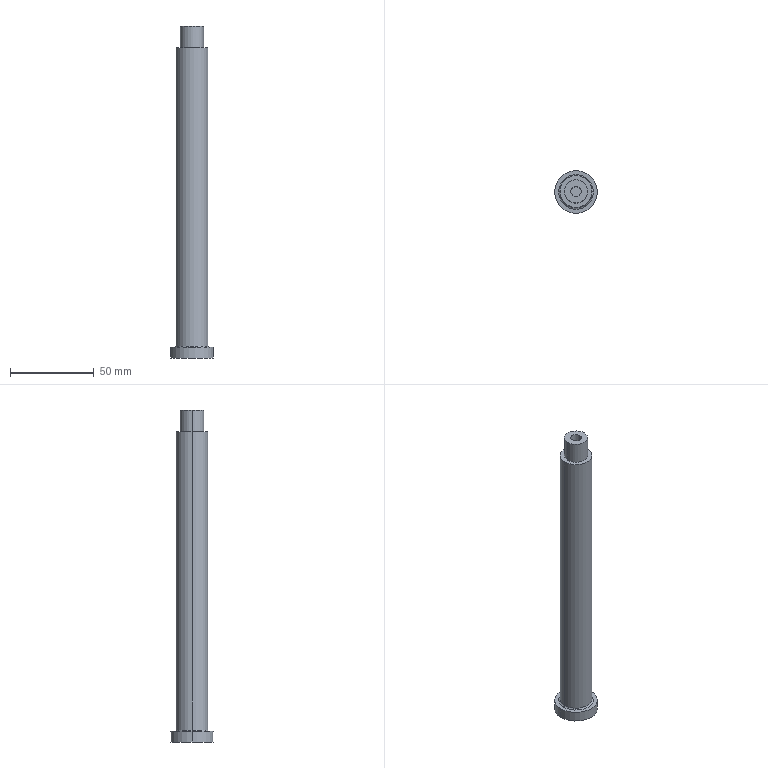Part | STEP file | 4-20.sldasm-Part-369 | 1 solid | 15 faces | box 25.4 x 25.4 x 198 mm | volume 50153 mm3 | cylinder 8 | plane 5 | torus 2 | commonest cylinder face diameters 6.35 x2 13.862 x2 19.05 x2 25.4 x2
STEP:
#1=CARTESIAN_POINT('',(5.825,320.,-95.));
#2=VERTEX_POINT('',#1);
#3=CARTESIAN_POINT('',(12.175,320.,-95.));
#4=VERTEX_POINT('',#3);
#5=CARTESIAN_POINT('',(9.,320.,-95.));
#6=DIRECTION('',(0.,0.,1.));
#7=DIRECTION('',(-1.,0.,0.));
#8=AXIS2_PLACEMENT_3D('',#5,#6,#7);
#9=CIRCLE('',#8,3.175);
#10=EDGE_CURVE('',#2,#4,#9,.T.);
#11=ORIENTED_EDGE('',*,*,#10,.F.);
#12=CARTESIAN_POINT('',(5.825,320.,93.));
#13=VERTEX_POINT('',#12);
#14=CARTESIAN_POINT('',(5.825,320.,-405.));
#15=DIRECTION('',(0.,0.,1.));
#16=VECTOR('',#15,1000.);
#17=LINE('',#14,#16);
#18=EDGE_CURVE('',#2,#13,#17,.T.);
#19=ORIENTED_EDGE('',*,*,#18,.T.);
#20=CARTESIAN_POINT('',(12.175,320.,93.));
#21=VERTEX_POINT('',#20);
#22=CARTESIAN_POINT('',(9.,320.,93.));
#23=DIRECTION('',(0.,0.,1.));
#24=DIRECTION('',(-1.,0.,0.));
#25=AXIS2_PLACEMENT_3D('',#22,#23,#24);
#26=CIRCLE('',#25,3.175);
#27=EDGE_CURVE('',#13,#21,#26,.T.);
#28=ORIENTED_EDGE('',*,*,#27,.T.);
#29=CARTESIAN_POINT('',(12.175,320.,-405.));
#30=DIRECTION('',(0.,0.,1.));
#31=VECTOR('',#30,1000.);
#32=LINE('',#29,#31);
#33=EDGE_CURVE('',#4,#21,#32,.T.);
#34=ORIENTED_EDGE('',*,*,#33,.F.);
#35=EDGE_LOOP('',(#11,#19,#28,#34));
#36=FACE_OUTER_BOUND('',#35,.T.);
#37=CARTESIAN_POINT('',(9.,320.,-405.));
#38=DIRECTION('',(0.,0.,1.));
#39=DIRECTION('',(1.,0.,0.));
#40=AXIS2_PLACEMENT_3D('',#37,#38,#39);
#41=CYLINDRICAL_SURFACE('',#40,3.175);
#42=ADVANCED_FACE('',(#36),#41,.F.);
#43=CARTESIAN_POINT('',(15.931,320.,93.));
#44=VERTEX_POINT('',#43);
#45=CARTESIAN_POINT('',(2.069,320.,93.));
#46=VERTEX_POINT('',#45);
#47=CARTESIAN_POINT('',(9.,320.,93.));
#48=DIRECTION('',(0.,0.,1.));
#49=DIRECTION('',(-1.,0.,0.));
#50=AXIS2_PLACEMENT_3D('',#47,#48,#49);
#51=CIRCLE('',#50,6.931);
#52=EDGE_CURVE('',#44,#46,#51,.T.);
#53=ORIENTED_EDGE('',*,*,#52,.F.);
#54=CARTESIAN_POINT('',(15.931,320.,80.));
#55=VERTEX_POINT('',#54);
#56=CARTESIAN_POINT('',(15.931,320.,62.4));
#57=DIRECTION('',(0.,0.,-1.));
#58=VECTOR('',#57,1000.);
#59=LINE('',#56,#58);
#60=EDGE_CURVE('',#44,#55,#59,.T.);
#61=ORIENTED_EDGE('',*,*,#60,.T.);
#62=CARTESIAN_POINT('',(2.069,320.,80.));
#63=VERTEX_POINT('',#62);
#64=CARTESIAN_POINT('',(9.,320.,80.));
#65=DIRECTION('',(0.,0.,1.));
#66=DIRECTION('',(1.,0.,0.));
#67=AXIS2_PLACEMENT_3D('',#64,#65,#66);
#68=CIRCLE('',#67,6.931);
#69=EDGE_CURVE('',#55,#63,#68,.T.);
#70=ORIENTED_EDGE('',*,*,#69,.T.);
#71=CARTESIAN_POINT('',(2.069,320.,62.4));
#72=DIRECTION('',(0.,0.,-1.));
#73=VECTOR('',#72,1000.);
#74=LINE('',#71,#73);
#75=EDGE_CURVE('',#46,#63,#74,.T.);
#76=ORIENTED_EDGE('',*,*,#75,.F.);
#77=EDGE_LOOP('',(#53,#61,#70,#76));
#78=FACE_OUTER_BOUND('',#77,.T.);
#79=CARTESIAN_POINT('',(9.,320.,62.4));
#80=DIRECTION('',(0.,0.,-1.));
#81=DIRECTION('',(-1.,0.,0.));
#82=AXIS2_PLACEMENT_3D('',#79,#80,#81);
#83=CYLINDRICAL_SURFACE('',#82,6.931);
#84=ADVANCED_FACE('',(#78),#83,.T.);
#85=CARTESIAN_POINT('',(-1.319,320.,-98.65));
#86=VERTEX_POINT('',#85);
#87=CARTESIAN_POINT('',(19.319,320.,-98.65));
#88=VERTEX_POINT('',#87);
#89=CARTESIAN_POINT('',(9.,320.,-98.65));
#90=DIRECTION('',(0.,0.,1.));
#91=DIRECTION('',(0.,-1.,0.));
#92=AXIS2_PLACEMENT_3D('',#89,#90,#91);
#93=CIRCLE('',#92,10.319);
#94=EDGE_CURVE('',#86,#88,#93,.T.);
#95=ORIENTED_EDGE('',*,*,#94,.T.);
#96=CARTESIAN_POINT('',(18.525,320.,-97.856));
#97=VERTEX_POINT('',#96);
#98=CARTESIAN_POINT('',(19.319,320.,-97.856));
#99=DIRECTION('',(0.,1.,0.));
#100=DIRECTION('',(-1.,0.,0.));
#101=AXIS2_PLACEMENT_3D('',#98,#99,#100);
#102=CIRCLE('',#101,0.7937);
#103=EDGE_CURVE('',#88,#97,#102,.T.);
#104=ORIENTED_EDGE('',*,*,#103,.T.);
#105=CARTESIAN_POINT('',(-0.525,320.,-97.856));
#106=VERTEX_POINT('',#105);
#107=CARTESIAN_POINT('',(9.,320.,-97.856));
#108=DIRECTION('',(0.,0.,1.));
#109=DIRECTION('',(0.,-1.,0.));
#110=AXIS2_PLACEMENT_3D('',#107,#108,#109);
#111=CIRCLE('',#110,9.525);
#112=EDGE_CURVE('',#106,#97,#111,.T.);
#113=ORIENTED_EDGE('',*,*,#112,.F.);
#114=CARTESIAN_POINT('',(-1.319,320.,-97.856));
#115=DIRECTION('',(0.,-1.,0.));
#116=DIRECTION('',(0.,0.,-1.));
#117=AXIS2_PLACEMENT_3D('',#114,#115,#116);
#118=CIRCLE('',#117,0.7937);
#119=EDGE_CURVE('',#86,#106,#118,.T.);
#120=ORIENTED_EDGE('',*,*,#119,.F.);
#121=EDGE_LOOP('',(#95,#104,#113,#120));
#122=FACE_OUTER_BOUND('',#121,.T.);
#123=CARTESIAN_POINT('',(9.,320.,-97.856));
#124=DIRECTION('',(0.,0.,-1.));
#125=DIRECTION('',(-1.,0.,0.));
#126=AXIS2_PLACEMENT_3D('',#123,#124,#125);
#127=TOROIDAL_SURFACE('',#126,10.319,0.7937);
#128=ADVANCED_FACE('',(#122),#127,.F.);
#129=CARTESIAN_POINT('',(21.7,320.,-105.));
#130=VERTEX_POINT('',#129);
#131=CARTESIAN_POINT('',(-3.7,320.,-105.));
#132=VERTEX_POINT('',#131);
#133=CARTESIAN_POINT('',(9.,320.,-105.));
#134=DIRECTION('',(0.,0.,1.));
#135=DIRECTION('',(0.,-1.,0.));
#136=AXIS2_PLACEMENT_3D('',#133,#134,#135);
#137=CIRCLE('',#136,12.7);
#138=EDGE_CURVE('',#130,#132,#137,.T.);
#139=ORIENTED_EDGE('',*,*,#138,.T.);
#140=CARTESIAN_POINT('',(-3.7,320.,-98.65));
#141=VERTEX_POINT('',#140);
#142=CARTESIAN_POINT('',(-3.7,320.,-101.825));
#143=DIRECTION('',(0.,0.,1.));
#144=VECTOR('',#143,1000.);
#145=LINE('',#142,#144);
#146=EDGE_CURVE('',#132,#141,#145,.T.);
#147=ORIENTED_EDGE('',*,*,#146,.T.);
#148=CARTESIAN_POINT('',(21.7,320.,-98.65));
#149=VERTEX_POINT('',#148);
#150=CARTESIAN_POINT('',(9.,320.,-98.65));
#151=DIRECTION('',(0.,0.,1.));
#152=DIRECTION('',(0.,-1.,0.));
#153=AXIS2_PLACEMENT_3D('',#150,#151,#152);
#154=CIRCLE('',#153,12.7);
#155=EDGE_CURVE('',#149,#141,#154,.T.);
#156=ORIENTED_EDGE('',*,*,#155,.F.);
#157=CARTESIAN_POINT('',(21.7,320.,-101.825));
#158=DIRECTION('',(0.,0.,1.));
#159=VECTOR('',#158,1000.);
#160=LINE('',#157,#159);
#161=EDGE_CURVE('',#130,#149,#160,.T.);
#162=ORIENTED_EDGE('',*,*,#161,.F.);
#163=EDGE_LOOP('',(#139,#147,#156,#162));
#164=FACE_OUTER_BOUND('',#163,.T.);
#165=CARTESIAN_POINT('',(9.,320.,-101.825));
#166=DIRECTION('',(0.,0.,1.));
#167=DIRECTION('',(1.,0.,0.));
#168=AXIS2_PLACEMENT_3D('',#165,#166,#167);
#169=CYLINDRICAL_SURFACE('',#168,12.7);
#170=ADVANCED_FACE('',(#164),#169,.T.);
#171=CARTESIAN_POINT('',(9.,320.,-97.856));
#172=DIRECTION('',(0.,0.,1.));
#173=DIRECTION('',(0.,-1.,0.));
#174=AXIS2_PLACEMENT_3D('',#171,#172,#173);
#175=CIRCLE('',#174,9.525);
#176=EDGE_CURVE('',#97,#106,#175,.T.);
#177=ORIENTED_EDGE('',*,*,#176,.T.);
#178=CARTESIAN_POINT('',(-0.525,320.,80.));
#179=VERTEX_POINT('',#178);
#180=CARTESIAN_POINT('',(-0.525,320.,-25.228));
#181=DIRECTION('',(0.,0.,1.));
#182=VECTOR('',#181,1000.);
#183=LINE('',#180,#182);
#184=EDGE_CURVE('',#106,#179,#183,.T.);
#185=ORIENTED_EDGE('',*,*,#184,.T.);
#186=CARTESIAN_POINT('',(18.525,320.,80.));
#187=VERTEX_POINT('',#186);
#188=CARTESIAN_POINT('',(9.,320.,80.));
#189=DIRECTION('',(0.,0.,1.));
#190=DIRECTION('',(1.,0.,0.));
#191=AXIS2_PLACEMENT_3D('',#188,#189,#190);
#192=CIRCLE('',#191,9.525);
#193=EDGE_CURVE('',#187,#179,#192,.T.);
#194=ORIENTED_EDGE('',*,*,#193,.F.);
#195=CARTESIAN_POINT('',(18.525,320.,-25.228));
#196=DIRECTION('',(0.,0.,1.));
#197=VECTOR('',#196,1000.);
#198=LINE('',#195,#197);
#199=EDGE_CURVE('',#97,#187,#198,.T.);
#200=ORIENTED_EDGE('',*,*,#199,.F.);
#201=EDGE_LOOP('',(#177,#185,#194,#200));
#202=FACE_OUTER_BOUND('',#201,.T.);
#203=CARTESIAN_POINT('',(9.,320.,-25.228));
#204=DIRECTION('',(0.,0.,1.));
#205=DIRECTION('',(1.,0.,0.));
#206=AXIS2_PLACEMENT_3D('',#203,#204,#205);
#207=CYLINDRICAL_SURFACE('',#206,9.525);
#208=ADVANCED_FACE('',(#202),#207,.T.);
#209=ORIENTED_EDGE('',*,*,#193,.T.);
#210=CARTESIAN_POINT('',(9.,320.,80.));
#211=DIRECTION('',(0.,0.,1.));
#212=DIRECTION('',(1.,0.,0.));
#213=AXIS2_PLACEMENT_3D('',#210,#211,#212);
#214=CIRCLE('',#213,9.525);
#215=EDGE_CURVE('',#179,#187,#214,.T.);
#216=ORIENTED_EDGE('',*,*,#215,.T.);
#217=EDGE_LOOP('',(#209,#216));
#218=FACE_OUTER_BOUND('',#217,.T.);
#219=CARTESIAN_POINT('',(9.,320.,80.));
#220=DIRECTION('',(0.,0.,1.));
#221=DIRECTION('',(1.,0.,0.));
#222=AXIS2_PLACEMENT_3D('',#219,#220,#221);
#223=CIRCLE('',#222,6.931);
#224=EDGE_CURVE('',#63,#55,#223,.T.);
#225=ORIENTED_EDGE('',*,*,#224,.F.);
#226=ORIENTED_EDGE('',*,*,#69,.F.);
#227=EDGE_LOOP('',(#225,#226));
#228=FACE_BOUND('',#227,.T.);
#229=CARTESIAN_POINT('',(9.,320.,80.));
#230=DIRECTION('',(0.,0.,1.));
#231=DIRECTION('',(1.,0.,0.));
#232=AXIS2_PLACEMENT_3D('',#229,#230,#231);
#233=PLANE('',#232);
#234=ADVANCED_FACE('',(#218,#228),#233,.T.);
#235=ORIENTED_EDGE('',*,*,#184,.F.);
#236=ORIENTED_EDGE('',*,*,#112,.T.);
#237=ORIENTED_EDGE('',*,*,#199,.T.);
#238=ORIENTED_EDGE('',*,*,#215,.F.);
#239=EDGE_LOOP('',(#235,#236,#237,#238));
#240=FACE_OUTER_BOUND('',#239,.T.);
#241=CARTESIAN_POINT('',(9.,320.,-25.228));
#242=DIRECTION('',(0.,0.,1.));
#243=DIRECTION('',(1.,0.,0.));
#244=AXIS2_PLACEMENT_3D('',#241,#242,#243);
#245=CYLINDRICAL_SURFACE('',#244,9.525);
#246=ADVANCED_FACE('',(#240),#245,.T.);
#247=ORIENTED_EDGE('',*,*,#138,.F.);
#248=CARTESIAN_POINT('',(9.,320.,-105.));
#249=DIRECTION('',(0.,0.,1.));
#250=DIRECTION('',(0.,-1.,0.));
#251=AXIS2_PLACEMENT_3D('',#248,#249,#250);
#252=CIRCLE('',#251,12.7);
#253=EDGE_CURVE('',#132,#130,#252,.T.);
#254=ORIENTED_EDGE('',*,*,#253,.F.);
#255=EDGE_LOOP('',(#247,#254));
#256=FACE_OUTER_BOUND('',#255,.T.);
#257=CARTESIAN_POINT('',(9.,313.65,-105.));
#258=DIRECTION('',(0.,0.,-1.));
#259=DIRECTION('',(-1.,0.,0.));
#260=AXIS2_PLACEMENT_3D('',#257,#258,#259);
#261=PLANE('',#260);
#262=ADVANCED_FACE('',(#256),#261,.T.);
#263=ORIENTED_EDGE('',*,*,#146,.F.);
#264=ORIENTED_EDGE('',*,*,#253,.T.);
#265=ORIENTED_EDGE('',*,*,#161,.T.);
#266=CARTESIAN_POINT('',(9.,320.,-98.65));
#267=DIRECTION('',(0.,0.,1.));
#268=DIRECTION('',(0.,-1.,0.));
#269=AXIS2_PLACEMENT_3D('',#266,#267,#268);
#270=CIRCLE('',#269,12.7);
#271=EDGE_CURVE('',#141,#149,#270,.T.);
#272=ORIENTED_EDGE('',*,*,#271,.F.);
#273=EDGE_LOOP('',(#263,#264,#265,#272));
#274=FACE_OUTER_BOUND('',#273,.T.);
#275=CARTESIAN_POINT('',(9.,320.,-101.825));
#276=DIRECTION('',(0.,0.,1.));
#277=DIRECTION('',(1.,0.,0.));
#278=AXIS2_PLACEMENT_3D('',#275,#276,#277);
#279=CYLINDRICAL_SURFACE('',#278,12.7);
#280=ADVANCED_FACE('',(#274),#279,.T.);
#281=ORIENTED_EDGE('',*,*,#103,.F.);
#282=CARTESIAN_POINT('',(9.,320.,-98.65));
#283=DIRECTION('',(0.,0.,1.));
#284=DIRECTION('',(0.,-1.,0.));
#285=AXIS2_PLACEMENT_3D('',#282,#283,#284);
#286=CIRCLE('',#285,10.319);
#287=EDGE_CURVE('',#88,#86,#286,.T.);
#288=ORIENTED_EDGE('',*,*,#287,.T.);
#289=ORIENTED_EDGE('',*,*,#119,.T.);
#290=ORIENTED_EDGE('',*,*,#176,.F.);
#291=EDGE_LOOP('',(#281,#288,#289,#290));
#292=FACE_OUTER_BOUND('',#291,.T.);
#293=CARTESIAN_POINT('',(9.,320.,-97.856));
#294=DIRECTION('',(0.,0.,-1.));
#295=DIRECTION('',(-1.,0.,0.));
#296=AXIS2_PLACEMENT_3D('',#293,#294,#295);
#297=TOROIDAL_SURFACE('',#296,10.319,0.7937);
#298=ADVANCED_FACE('',(#292),#297,.F.);
#299=ORIENTED_EDGE('',*,*,#155,.T.);
#300=ORIENTED_EDGE('',*,*,#271,.T.);
#301=EDGE_LOOP('',(#299,#300));
#302=FACE_OUTER_BOUND('',#301,.T.);
#303=ORIENTED_EDGE('',*,*,#94,.F.);
#304=ORIENTED_EDGE('',*,*,#287,.F.);
#305=EDGE_LOOP('',(#303,#304));
#306=FACE_BOUND('',#305,.T.);
#307=CARTESIAN_POINT('',(9.,308.491,-98.65));
#308=DIRECTION('',(0.,0.,1.));
#309=DIRECTION('',(1.,0.,0.));
#310=AXIS2_PLACEMENT_3D('',#307,#308,#309);
#311=PLANE('',#310);
#312=ADVANCED_FACE('',(#302,#306),#311,.T.);
#313=ORIENTED_EDGE('',*,*,#60,.F.);
#314=CARTESIAN_POINT('',(9.,320.,93.));
#315=DIRECTION('',(0.,0.,1.));
#316=DIRECTION('',(-1.,0.,0.));
#317=AXIS2_PLACEMENT_3D('',#314,#315,#316);
#318=CIRCLE('',#317,6.931);
#319=EDGE_CURVE('',#46,#44,#318,.T.);
#320=ORIENTED_EDGE('',*,*,#319,.F.);
#321=ORIENTED_EDGE('',*,*,#75,.T.);
#322=ORIENTED_EDGE('',*,*,#224,.T.);
#323=EDGE_LOOP('',(#313,#320,#321,#322));
#324=FACE_OUTER_BOUND('',#323,.T.);
#325=CARTESIAN_POINT('',(9.,320.,62.4));
#326=DIRECTION('',(0.,0.,-1.));
#327=DIRECTION('',(-1.,0.,0.));
#328=AXIS2_PLACEMENT_3D('',#325,#326,#327);
#329=CYLINDRICAL_SURFACE('',#328,6.931);
#330=ADVANCED_FACE('',(#324),#329,.T.);
#331=ORIENTED_EDGE('',*,*,#319,.T.);
#332=ORIENTED_EDGE('',*,*,#52,.T.);
#333=EDGE_LOOP('',(#331,#332));
#334=FACE_OUTER_BOUND('',#333,.T.);
#335=CARTESIAN_POINT('',(9.,320.,93.));
#336=DIRECTION('',(0.,0.,1.));
#337=DIRECTION('',(-1.,0.,0.));
#338=AXIS2_PLACEMENT_3D('',#335,#336,#337);
#339=CIRCLE('',#338,3.175);
#340=EDGE_CURVE('',#21,#13,#339,.T.);
#341=ORIENTED_EDGE('',*,*,#340,.F.);
#342=ORIENTED_EDGE('',*,*,#27,.F.);
#343=EDGE_LOOP('',(#341,#342));
#344=FACE_BOUND('',#343,.T.);
#345=CARTESIAN_POINT('',(9.,0.,93.));
#346=DIRECTION('',(0.,0.,-1.));
#347=DIRECTION('',(-1.,0.,0.));
#348=AXIS2_PLACEMENT_3D('',#345,#346,#347);
#349=PLANE('',#348);
#350=ADVANCED_FACE('',(#334,#344),#349,.F.);
#351=CARTESIAN_POINT('',(9.,320.,-95.));
#352=DIRECTION('',(0.,0.,1.));
#353=DIRECTION('',(-1.,0.,0.));
#354=AXIS2_PLACEMENT_3D('',#351,#352,#353);
#355=CIRCLE('',#354,3.175);
#356=EDGE_CURVE('',#4,#2,#355,.T.);
#357=ORIENTED_EDGE('',*,*,#356,.T.);
#358=ORIENTED_EDGE('',*,*,#10,.T.);
#359=EDGE_LOOP('',(#357,#358));
#360=FACE_OUTER_BOUND('',#359,.T.);
#361=CARTESIAN_POINT('',(9.,320.,-95.));
#362=DIRECTION('',(0.,0.,-1.));
#363=DIRECTION('',(-1.,0.,0.));
#364=AXIS2_PLACEMENT_3D('',#361,#362,#363);
#365=PLANE('',#364);
#366=ADVANCED_FACE('',(#360),#365,.F.);
#367=ORIENTED_EDGE('',*,*,#18,.F.);
#368=ORIENTED_EDGE('',*,*,#356,.F.);
#369=ORIENTED_EDGE('',*,*,#33,.T.);
#370=ORIENTED_EDGE('',*,*,#340,.T.);
#371=EDGE_LOOP('',(#367,#368,#369,#370));
#372=FACE_OUTER_BOUND('',#371,.T.);
#373=CARTESIAN_POINT('',(9.,320.,-405.));
#374=DIRECTION('',(0.,0.,1.));
#375=DIRECTION('',(1.,0.,0.));
#376=AXIS2_PLACEMENT_3D('',#373,#374,#375);
#377=CYLINDRICAL_SURFACE('',#376,3.175);
#378=ADVANCED_FACE('',(#372),#377,.F.);
#379=CLOSED_SHELL('',(#42,#84,#128,#170,#208,#234,#246,#262,#280,#298,#312,#330,#350,#366,#378));
#380=MANIFOLD_SOLID_BREP('',#379);
#381=CARTESIAN_POINT('',(0.,0.,0.));
#382=DIRECTION('',(0.,0.,1.));
#383=DIRECTION('',(1.,0.,0.));
#384=AXIS2_PLACEMENT_3D('',#381,#382,#383);
#385=(LENGTH_UNIT()NAMED_UNIT(*)SI_UNIT(.MILLI.,.METRE.));
#386=UNCERTAINTY_MEASURE_WITH_UNIT(LENGTH_MEASURE(0.00001),#385,'','');
#387=(NAMED_UNIT(*)PLANE_ANGLE_UNIT()SI_UNIT($,.RADIAN.));
#388=(NAMED_UNIT(*)SI_UNIT($,.STERADIAN.)SOLID_ANGLE_UNIT());
#389=(GEOMETRIC_REPRESENTATION_CONTEXT(3)GLOBAL_UNCERTAINTY_ASSIGNED_CONTEXT((#386))GLOBAL_UNIT_ASSIGNED_CONTEXT((#385,#387,#388))REPRESENTATION_CONTEXT('',''));
#390=ADVANCED_BREP_SHAPE_REPRESENTATION('',(#380,#384),#389);